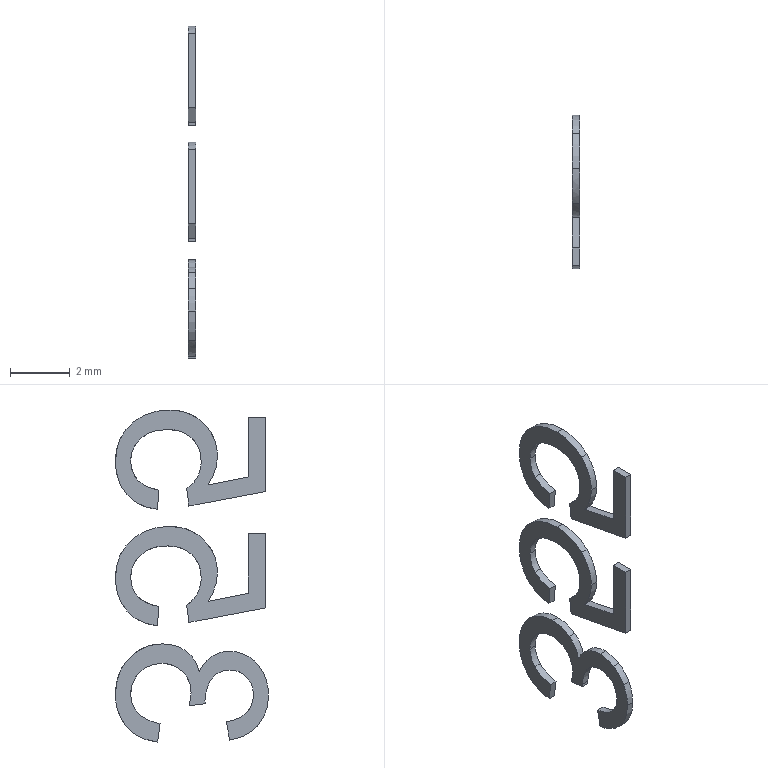Part | STEP file | BBS-JK-ZYBL-355-H5-1.stp.STEP | 3 solids | 80 faces | box 0.25 x 5.109 x 11.081 mm | volume 5.038 mm3 | spline 57 | plane 23